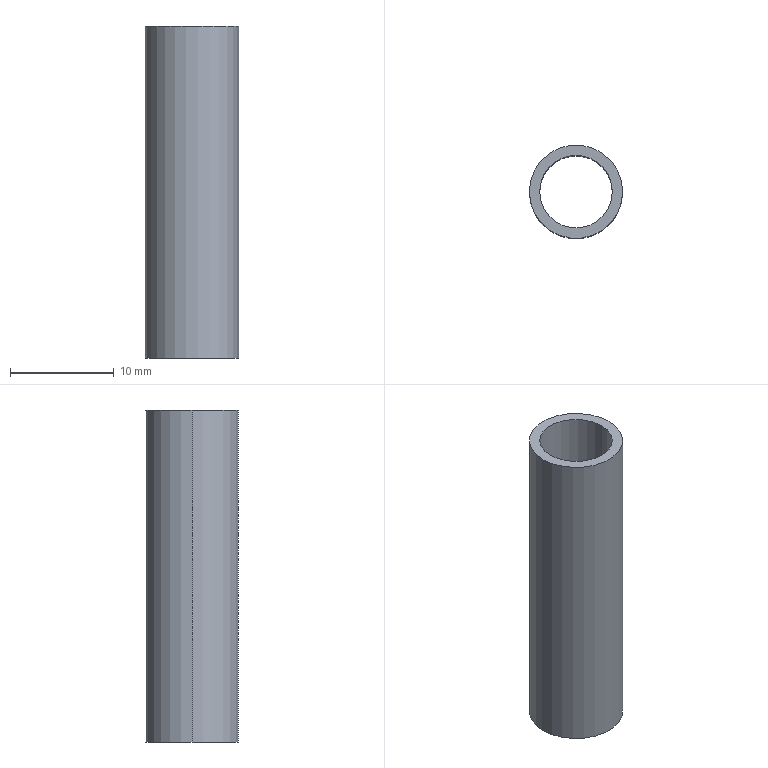Part | SolidWorks | features Extrusion 1 | 1 solid | 6 faces | box 9 x 9 x 32 mm | volume 804.248 mm3 | cylinder 4 | plane 2 | commonest cylinder face diameters 7 x2 9 x2
STEP:
#1=CARTESIAN_POINT('',(-3.5,0.,32.));
#2=VERTEX_POINT('',#1);
#3=CARTESIAN_POINT('',(3.5,0.,32.));
#4=VERTEX_POINT('',#3);
#5=CARTESIAN_POINT('',(0.,0.,32.));
#6=DIRECTION('',(0.,0.,1.));
#7=DIRECTION('',(1.,0.,0.));
#8=AXIS2_PLACEMENT_3D('',#5,#6,#7);
#9=CIRCLE('',#8,3.5);
#10=EDGE_CURVE('',#2,#4,#9,.T.);
#11=ORIENTED_EDGE('',*,*,#10,.T.);
#12=CARTESIAN_POINT('',(3.5,0.,0.));
#13=VERTEX_POINT('',#12);
#14=CARTESIAN_POINT('',(3.5,0.,32.));
#15=DIRECTION('',(0.,0.,-1.));
#16=VECTOR('',#15,1000.);
#17=LINE('',#14,#16);
#18=EDGE_CURVE('',#4,#13,#17,.T.);
#19=ORIENTED_EDGE('',*,*,#18,.T.);
#20=CARTESIAN_POINT('',(-3.5,0.,0.));
#21=VERTEX_POINT('',#20);
#22=CARTESIAN_POINT('',(0.,0.,0.));
#23=DIRECTION('',(0.,0.,1.));
#24=DIRECTION('',(1.,0.,0.));
#25=AXIS2_PLACEMENT_3D('',#22,#23,#24);
#26=CIRCLE('',#25,3.5);
#27=EDGE_CURVE('',#21,#13,#26,.T.);
#28=ORIENTED_EDGE('',*,*,#27,.F.);
#29=CARTESIAN_POINT('',(-3.5,0.,32.));
#30=DIRECTION('',(0.,0.,-1.));
#31=VECTOR('',#30,1000.);
#32=LINE('',#29,#31);
#33=EDGE_CURVE('',#2,#21,#32,.T.);
#34=ORIENTED_EDGE('',*,*,#33,.F.);
#35=EDGE_LOOP('',(#11,#19,#28,#34));
#36=FACE_OUTER_BOUND('',#35,.T.);
#37=CARTESIAN_POINT('',(0.,0.,32.));
#38=DIRECTION('',(0.,0.,-1.));
#39=DIRECTION('',(-1.,0.,0.));
#40=AXIS2_PLACEMENT_3D('',#37,#38,#39);
#41=CYLINDRICAL_SURFACE('',#40,3.5);
#42=ADVANCED_FACE('',(#36),#41,.F.);
#43=CARTESIAN_POINT('',(4.5,0.,32.));
#44=VERTEX_POINT('',#43);
#45=CARTESIAN_POINT('',(-4.5,0.,32.));
#46=VERTEX_POINT('',#45);
#47=CARTESIAN_POINT('',(0.,0.,32.));
#48=DIRECTION('',(0.,0.,1.));
#49=DIRECTION('',(1.,0.,0.));
#50=AXIS2_PLACEMENT_3D('',#47,#48,#49);
#51=CIRCLE('',#50,4.5);
#52=EDGE_CURVE('',#44,#46,#51,.T.);
#53=ORIENTED_EDGE('',*,*,#52,.F.);
#54=CARTESIAN_POINT('',(4.5,0.,0.));
#55=VERTEX_POINT('',#54);
#56=CARTESIAN_POINT('',(4.5,0.,32.));
#57=DIRECTION('',(0.,0.,-1.));
#58=VECTOR('',#57,1000.);
#59=LINE('',#56,#58);
#60=EDGE_CURVE('',#44,#55,#59,.T.);
#61=ORIENTED_EDGE('',*,*,#60,.T.);
#62=CARTESIAN_POINT('',(-4.5,0.,0.));
#63=VERTEX_POINT('',#62);
#64=CARTESIAN_POINT('',(0.,0.,0.));
#65=DIRECTION('',(0.,0.,1.));
#66=DIRECTION('',(1.,0.,0.));
#67=AXIS2_PLACEMENT_3D('',#64,#65,#66);
#68=CIRCLE('',#67,4.5);
#69=EDGE_CURVE('',#55,#63,#68,.T.);
#70=ORIENTED_EDGE('',*,*,#69,.T.);
#71=CARTESIAN_POINT('',(-4.5,0.,32.));
#72=DIRECTION('',(0.,0.,-1.));
#73=VECTOR('',#72,1000.);
#74=LINE('',#71,#73);
#75=EDGE_CURVE('',#46,#63,#74,.T.);
#76=ORIENTED_EDGE('',*,*,#75,.F.);
#77=EDGE_LOOP('',(#53,#61,#70,#76));
#78=FACE_OUTER_BOUND('',#77,.T.);
#79=CARTESIAN_POINT('',(0.,0.,32.));
#80=DIRECTION('',(0.,0.,-1.));
#81=DIRECTION('',(-1.,0.,0.));
#82=AXIS2_PLACEMENT_3D('',#79,#80,#81);
#83=CYLINDRICAL_SURFACE('',#82,4.5);
#84=ADVANCED_FACE('',(#78),#83,.T.);
#85=CARTESIAN_POINT('',(0.,0.,32.));
#86=DIRECTION('',(0.,0.,1.));
#87=DIRECTION('',(1.,0.,0.));
#88=AXIS2_PLACEMENT_3D('',#85,#86,#87);
#89=CIRCLE('',#88,4.5);
#90=EDGE_CURVE('',#46,#44,#89,.T.);
#91=ORIENTED_EDGE('',*,*,#90,.T.);
#92=ORIENTED_EDGE('',*,*,#52,.T.);
#93=EDGE_LOOP('',(#91,#92));
#94=FACE_OUTER_BOUND('',#93,.T.);
#95=ORIENTED_EDGE('',*,*,#10,.F.);
#96=CARTESIAN_POINT('',(0.,0.,32.));
#97=DIRECTION('',(0.,0.,1.));
#98=DIRECTION('',(1.,0.,0.));
#99=AXIS2_PLACEMENT_3D('',#96,#97,#98);
#100=CIRCLE('',#99,3.5);
#101=EDGE_CURVE('',#4,#2,#100,.T.);
#102=ORIENTED_EDGE('',*,*,#101,.F.);
#103=EDGE_LOOP('',(#95,#102));
#104=FACE_BOUND('',#103,.T.);
#105=CARTESIAN_POINT('',(0.,0.,32.));
#106=DIRECTION('',(0.,0.,1.));
#107=DIRECTION('',(1.,0.,0.));
#108=AXIS2_PLACEMENT_3D('',#105,#106,#107);
#109=PLANE('',#108);
#110=ADVANCED_FACE('',(#94,#104),#109,.T.);
#111=CARTESIAN_POINT('',(0.,0.,0.));
#112=DIRECTION('',(0.,0.,1.));
#113=DIRECTION('',(1.,0.,0.));
#114=AXIS2_PLACEMENT_3D('',#111,#112,#113);
#115=CIRCLE('',#114,4.5);
#116=EDGE_CURVE('',#63,#55,#115,.T.);
#117=ORIENTED_EDGE('',*,*,#116,.F.);
#118=ORIENTED_EDGE('',*,*,#69,.F.);
#119=EDGE_LOOP('',(#117,#118));
#120=FACE_OUTER_BOUND('',#119,.T.);
#121=ORIENTED_EDGE('',*,*,#27,.T.);
#122=CARTESIAN_POINT('',(0.,0.,0.));
#123=DIRECTION('',(0.,0.,1.));
#124=DIRECTION('',(1.,0.,0.));
#125=AXIS2_PLACEMENT_3D('',#122,#123,#124);
#126=CIRCLE('',#125,3.5);
#127=EDGE_CURVE('',#13,#21,#126,.T.);
#128=ORIENTED_EDGE('',*,*,#127,.T.);
#129=EDGE_LOOP('',(#121,#128));
#130=FACE_BOUND('',#129,.T.);
#131=CARTESIAN_POINT('',(0.,0.,0.));
#132=DIRECTION('',(0.,0.,1.));
#133=DIRECTION('',(1.,0.,0.));
#134=AXIS2_PLACEMENT_3D('',#131,#132,#133);
#135=PLANE('',#134);
#136=ADVANCED_FACE('',(#120,#130),#135,.F.);
#137=ORIENTED_EDGE('',*,*,#60,.F.);
#138=ORIENTED_EDGE('',*,*,#90,.F.);
#139=ORIENTED_EDGE('',*,*,#75,.T.);
#140=ORIENTED_EDGE('',*,*,#116,.T.);
#141=EDGE_LOOP('',(#137,#138,#139,#140));
#142=FACE_OUTER_BOUND('',#141,.T.);
#143=CARTESIAN_POINT('',(0.,0.,32.));
#144=DIRECTION('',(0.,0.,-1.));
#145=DIRECTION('',(-1.,0.,0.));
#146=AXIS2_PLACEMENT_3D('',#143,#144,#145);
#147=CYLINDRICAL_SURFACE('',#146,4.5);
#148=ADVANCED_FACE('',(#142),#147,.T.);
#149=ORIENTED_EDGE('',*,*,#18,.F.);
#150=ORIENTED_EDGE('',*,*,#101,.T.);
#151=ORIENTED_EDGE('',*,*,#33,.T.);
#152=ORIENTED_EDGE('',*,*,#127,.F.);
#153=EDGE_LOOP('',(#149,#150,#151,#152));
#154=FACE_OUTER_BOUND('',#153,.T.);
#155=CARTESIAN_POINT('',(0.,0.,32.));
#156=DIRECTION('',(0.,0.,-1.));
#157=DIRECTION('',(-1.,0.,0.));
#158=AXIS2_PLACEMENT_3D('',#155,#156,#157);
#159=CYLINDRICAL_SURFACE('',#158,3.5);
#160=ADVANCED_FACE('',(#154),#159,.F.);
#161=CLOSED_SHELL('',(#42,#84,#110,#136,#148,#160));
#162=MANIFOLD_SOLID_BREP('',#161);
#163=CARTESIAN_POINT('',(0.,0.,0.));
#164=DIRECTION('',(0.,0.,1.));
#165=DIRECTION('',(1.,0.,0.));
#166=AXIS2_PLACEMENT_3D('',#163,#164,#165);
#167=(LENGTH_UNIT()NAMED_UNIT(*)SI_UNIT(.MILLI.,.METRE.));
#168=UNCERTAINTY_MEASURE_WITH_UNIT(LENGTH_MEASURE(0.00001),#167,'','');
#169=(NAMED_UNIT(*)PLANE_ANGLE_UNIT()SI_UNIT($,.RADIAN.));
#170=(NAMED_UNIT(*)SI_UNIT($,.STERADIAN.)SOLID_ANGLE_UNIT());
#171=(GEOMETRIC_REPRESENTATION_CONTEXT(3)GLOBAL_UNCERTAINTY_ASSIGNED_CONTEXT((#168))GLOBAL_UNIT_ASSIGNED_CONTEXT((#167,#169,#170))REPRESENTATION_CONTEXT('',''));
#172=ADVANCED_BREP_SHAPE_REPRESENTATION('',(#162,#166),#171);